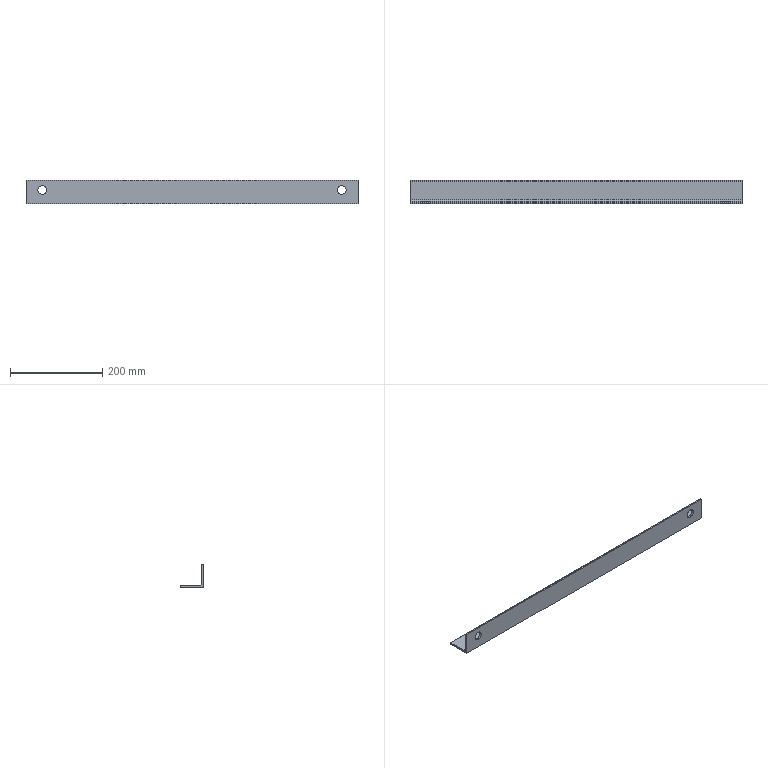Part | STEP file | 休息台角钢1_Default<As Machined> | 1 solid | 15 faces | box 721.5 x 50 x 50 mm | volume 278924 mm3 | plane 8 | cylinder 7 | commonest cylinder face diameters 19 x4 2.66 x2 11 x1
STEP:
#1=CARTESIAN_POINT('',(0.,0.,0.));
#2=DIRECTION('',(0.,0.,1.));
#3=DIRECTION('',(1.,0.,0.));
#4=AXIS2_PLACEMENT_3D('',#1,#2,#3);
#5=CARTESIAN_POINT('',(-325.75,0.,38.585));
#6=VERTEX_POINT('',#5);
#7=CARTESIAN_POINT('',(-325.75,4.,38.585));
#8=VERTEX_POINT('',#7);
#9=CARTESIAN_POINT('',(-325.75,-6.,38.585));
#10=DIRECTION('',(0.,1.,0.));
#11=VECTOR('',#10,1.);
#12=LINE('',#9,#11);
#13=CARTESIAN_POINT('',(-325.75,-6.,29.085));
#14=DIRECTION('',(0.,1.,0.));
#15=DIRECTION('',(0.,0.,1.));
#16=AXIS2_PLACEMENT_3D('',#13,#14,#15);
#17=CYLINDRICAL_SURFACE('',#16,9.5);
#18=CARTESIAN_POINT('',(6.283,0.));
#19=DIRECTION('',(0.,1.));
#20=VECTOR('',#19,1.);
#21=LINE('',#18,#20);
#22=(GEOMETRIC_REPRESENTATION_CONTEXT(2)PARAMETRIC_REPRESENTATION_CONTEXT()REPRESENTATION_CONTEXT('',''));
#23=DEFINITIONAL_REPRESENTATION('',(#21),#22);
#24=PCURVE('',#17,#23);
#25=CARTESIAN_POINT('',(-325.75,-6.,29.085));
#26=DIRECTION('',(0.,1.,0.));
#27=DIRECTION('',(0.,0.,1.));
#28=AXIS2_PLACEMENT_3D('',#25,#26,#27);
#29=CYLINDRICAL_SURFACE('',#28,9.5);
#30=CARTESIAN_POINT('',(0.,0.));
#31=DIRECTION('',(0.,1.));
#32=VECTOR('',#31,1.);
#33=LINE('',#30,#32);
#34=(GEOMETRIC_REPRESENTATION_CONTEXT(2)PARAMETRIC_REPRESENTATION_CONTEXT()REPRESENTATION_CONTEXT('',''));
#35=DEFINITIONAL_REPRESENTATION('',(#33),#34);
#36=PCURVE('',#29,#35);
#37=SURFACE_CURVE('',#12,(#24,#36),.PCURVE_S1.);
#38=EDGE_CURVE('',#6,#8,#37,.T.);
#39=ORIENTED_EDGE('',*,*,#38,.T.);
#40=CARTESIAN_POINT('',(-325.75,4.,19.585));
#41=VERTEX_POINT('',#40);
#42=CARTESIAN_POINT('',(-325.75,4.,29.085));
#43=DIRECTION('',(0.,1.,0.));
#44=DIRECTION('',(0.,0.,1.));
#45=AXIS2_PLACEMENT_3D('',#42,#43,#44);
#46=CIRCLE('',#45,9.5);
#47=CARTESIAN_POINT('',(0.,10.));
#48=DIRECTION('',(1.,0.));
#49=VECTOR('',#48,1.);
#50=LINE('',#47,#49);
#51=(GEOMETRIC_REPRESENTATION_CONTEXT(2)PARAMETRIC_REPRESENTATION_CONTEXT()REPRESENTATION_CONTEXT('',''));
#52=DEFINITIONAL_REPRESENTATION('',(#50),#51);
#53=PCURVE('',#17,#52);
#54=CARTESIAN_POINT('',(360.75,4.,48.67));
#55=DIRECTION('',(0.,-1.,0.));
#56=DIRECTION('',(1.,0.,0.));
#57=AXIS2_PLACEMENT_3D('',#54,#55,#56);
#58=PLANE('',#57);
#59=CARTESIAN_POINT('',(-686.5,-10.085));
#60=CARTESIAN_POINT('',(-670.046,-10.085));
#61=CARTESIAN_POINT('',(-678.273,-24.335));
#62=CARTESIAN_POINT('',(-686.5,-38.585));
#63=CARTESIAN_POINT('',(-694.727,-24.335));
#64=CARTESIAN_POINT('',(-702.954,-10.085));
#65=CARTESIAN_POINT('',(-686.5,-10.085));
#66=(BOUNDED_CURVE()B_SPLINE_CURVE(2,(#59,#60,#61,#62,#63,#64,#65),.UNSPECIFIED.,.T.,.F.)B_SPLINE_CURVE_WITH_KNOTS((1,2,2,2,2,1),(-2.094,0.,2.094,4.189,6.283,8.378),.UNSPECIFIED.)CURVE()GEOMETRIC_REPRESENTATION_ITEM()RATIONAL_B_SPLINE_CURVE((1.,0.5,1.,0.5,1.,0.5,1.))REPRESENTATION_ITEM(''));
#67=(GEOMETRIC_REPRESENTATION_CONTEXT(2)PARAMETRIC_REPRESENTATION_CONTEXT()REPRESENTATION_CONTEXT('',''));
#68=DEFINITIONAL_REPRESENTATION('',(#66),#67);
#69=PCURVE('',#58,#68);
#70=SURFACE_CURVE('',#46,(#53,#69),.PCURVE_S1.);
#71=EDGE_CURVE('',#41,#8,#70,.T.);
#72=ORIENTED_EDGE('',*,*,#71,.F.);
#73=CARTESIAN_POINT('',(-325.75,0.,19.585));
#74=VERTEX_POINT('',#73);
#75=CARTESIAN_POINT('',(-325.75,-6.,19.585));
#76=DIRECTION('',(0.,1.,0.));
#77=VECTOR('',#76,1.);
#78=LINE('',#75,#77);
#79=CARTESIAN_POINT('',(3.142,0.));
#80=DIRECTION('',(0.,1.));
#81=VECTOR('',#80,1.);
#82=LINE('',#79,#81);
#83=(GEOMETRIC_REPRESENTATION_CONTEXT(2)PARAMETRIC_REPRESENTATION_CONTEXT()REPRESENTATION_CONTEXT('',''));
#84=DEFINITIONAL_REPRESENTATION('',(#82),#83);
#85=PCURVE('',#17,#84);
#86=CARTESIAN_POINT('',(3.142,0.));
#87=DIRECTION('',(0.,1.));
#88=VECTOR('',#87,1.);
#89=LINE('',#86,#88);
#90=(GEOMETRIC_REPRESENTATION_CONTEXT(2)PARAMETRIC_REPRESENTATION_CONTEXT()REPRESENTATION_CONTEXT('',''));
#91=DEFINITIONAL_REPRESENTATION('',(#89),#90);
#92=PCURVE('',#29,#91);
#93=SURFACE_CURVE('',#78,(#85,#92),.PCURVE_S1.);
#94=EDGE_CURVE('',#74,#41,#93,.T.);
#95=ORIENTED_EDGE('',*,*,#94,.F.);
#96=CARTESIAN_POINT('',(-325.75,0.,29.085));
#97=DIRECTION('',(0.,1.,0.));
#98=DIRECTION('',(-1.,0.,0.));
#99=AXIS2_PLACEMENT_3D('',#96,#97,#98);
#100=CIRCLE('',#99,9.5);
#101=CARTESIAN_POINT('',(-1.571,6.));
#102=DIRECTION('',(1.,0.));
#103=VECTOR('',#102,1.);
#104=LINE('',#101,#103);
#105=(GEOMETRIC_REPRESENTATION_CONTEXT(2)PARAMETRIC_REPRESENTATION_CONTEXT()REPRESENTATION_CONTEXT('',''));
#106=DEFINITIONAL_REPRESENTATION('',(#104),#105);
#107=PCURVE('',#17,#106);
#108=CARTESIAN_POINT('',(360.75,0.,50.));
#109=DIRECTION('',(0.,1.,0.));
#110=DIRECTION('',(-1.,0.,0.));
#111=AXIS2_PLACEMENT_3D('',#108,#109,#110);
#112=PLANE('',#111);
#113=CARTESIAN_POINT('',(686.5,-20.915));
#114=DIRECTION('',(1.,0.));
#115=AXIS2_PLACEMENT_2D('',#113,#114);
#116=CIRCLE('',#115,9.5);
#117=(GEOMETRIC_REPRESENTATION_CONTEXT(2)PARAMETRIC_REPRESENTATION_CONTEXT()REPRESENTATION_CONTEXT('',''));
#118=DEFINITIONAL_REPRESENTATION('',(#116),#117);
#119=PCURVE('',#112,#118);
#120=SURFACE_CURVE('',#100,(#107,#119),.PCURVE_S1.);
#121=EDGE_CURVE('',#74,#6,#120,.T.);
#122=ORIENTED_EDGE('',*,*,#121,.T.);
#123=EDGE_LOOP('',(#39,#72,#95,#122));
#124=FACE_BOUND('',#123,.F.);
#125=ADVANCED_FACE('',(#124),#17,.F.);
#126=CARTESIAN_POINT('',(325.75,0.,38.585));
#127=VERTEX_POINT('',#126);
#128=CARTESIAN_POINT('',(325.75,4.,38.585));
#129=VERTEX_POINT('',#128);
#130=CARTESIAN_POINT('',(325.75,-6.,38.585));
#131=DIRECTION('',(0.,1.,0.));
#132=VECTOR('',#131,1.);
#133=LINE('',#130,#132);
#134=CARTESIAN_POINT('',(325.75,-6.,29.085));
#135=DIRECTION('',(0.,1.,0.));
#136=DIRECTION('',(0.,0.,1.));
#137=AXIS2_PLACEMENT_3D('',#134,#135,#136);
#138=CYLINDRICAL_SURFACE('',#137,9.5);
#139=CARTESIAN_POINT('',(6.283,0.));
#140=DIRECTION('',(0.,1.));
#141=VECTOR('',#140,1.);
#142=LINE('',#139,#141);
#143=(GEOMETRIC_REPRESENTATION_CONTEXT(2)PARAMETRIC_REPRESENTATION_CONTEXT()REPRESENTATION_CONTEXT('',''));
#144=DEFINITIONAL_REPRESENTATION('',(#142),#143);
#145=PCURVE('',#138,#144);
#146=CARTESIAN_POINT('',(325.75,-6.,29.085));
#147=DIRECTION('',(0.,1.,0.));
#148=DIRECTION('',(0.,0.,1.));
#149=AXIS2_PLACEMENT_3D('',#146,#147,#148);
#150=CYLINDRICAL_SURFACE('',#149,9.5);
#151=CARTESIAN_POINT('',(0.,0.));
#152=DIRECTION('',(0.,1.));
#153=VECTOR('',#152,1.);
#154=LINE('',#151,#153);
#155=(GEOMETRIC_REPRESENTATION_CONTEXT(2)PARAMETRIC_REPRESENTATION_CONTEXT()REPRESENTATION_CONTEXT('',''));
#156=DEFINITIONAL_REPRESENTATION('',(#154),#155);
#157=PCURVE('',#150,#156);
#158=SURFACE_CURVE('',#133,(#145,#157),.PCURVE_S1.);
#159=EDGE_CURVE('',#127,#129,#158,.T.);
#160=ORIENTED_EDGE('',*,*,#159,.T.);
#161=CARTESIAN_POINT('',(325.75,4.,19.585));
#162=VERTEX_POINT('',#161);
#163=CARTESIAN_POINT('',(325.75,4.,29.085));
#164=DIRECTION('',(0.,1.,0.));
#165=DIRECTION('',(0.,0.,-1.));
#166=AXIS2_PLACEMENT_3D('',#163,#164,#165);
#167=CIRCLE('',#166,9.5);
#168=CARTESIAN_POINT('',(3.142,10.));
#169=DIRECTION('',(1.,0.));
#170=VECTOR('',#169,1.);
#171=LINE('',#168,#170);
#172=(GEOMETRIC_REPRESENTATION_CONTEXT(2)PARAMETRIC_REPRESENTATION_CONTEXT()REPRESENTATION_CONTEXT('',''));
#173=DEFINITIONAL_REPRESENTATION('',(#171),#172);
#174=PCURVE('',#138,#173);
#175=CARTESIAN_POINT('',(-35.,-29.085));
#176=CARTESIAN_POINT('',(-51.454,-29.085));
#177=CARTESIAN_POINT('',(-43.227,-14.835));
#178=CARTESIAN_POINT('',(-35.,-0.585));
#179=CARTESIAN_POINT('',(-26.773,-14.835));
#180=CARTESIAN_POINT('',(-18.546,-29.085));
#181=CARTESIAN_POINT('',(-35.,-29.085));
#182=(BOUNDED_CURVE()B_SPLINE_CURVE(2,(#175,#176,#177,#178,#179,#180,#181),.UNSPECIFIED.,.T.,.F.)B_SPLINE_CURVE_WITH_KNOTS((1,2,2,2,2,1),(-2.094,0.,2.094,4.189,6.283,8.378),.UNSPECIFIED.)CURVE()GEOMETRIC_REPRESENTATION_ITEM()RATIONAL_B_SPLINE_CURVE((1.,0.5,1.,0.5,1.,0.5,1.))REPRESENTATION_ITEM(''));
#183=(GEOMETRIC_REPRESENTATION_CONTEXT(2)PARAMETRIC_REPRESENTATION_CONTEXT()REPRESENTATION_CONTEXT('',''));
#184=DEFINITIONAL_REPRESENTATION('',(#182),#183);
#185=PCURVE('',#58,#184);
#186=SURFACE_CURVE('',#167,(#174,#185),.PCURVE_S1.);
#187=EDGE_CURVE('',#162,#129,#186,.T.);
#188=ORIENTED_EDGE('',*,*,#187,.F.);
#189=CARTESIAN_POINT('',(325.75,0.,19.585));
#190=VERTEX_POINT('',#189);
#191=CARTESIAN_POINT('',(325.75,-6.,19.585));
#192=DIRECTION('',(0.,1.,0.));
#193=VECTOR('',#192,1.);
#194=LINE('',#191,#193);
#195=CARTESIAN_POINT('',(3.142,0.));
#196=DIRECTION('',(0.,1.));
#197=VECTOR('',#196,1.);
#198=LINE('',#195,#197);
#199=(GEOMETRIC_REPRESENTATION_CONTEXT(2)PARAMETRIC_REPRESENTATION_CONTEXT()REPRESENTATION_CONTEXT('',''));
#200=DEFINITIONAL_REPRESENTATION('',(#198),#199);
#201=PCURVE('',#138,#200);
#202=CARTESIAN_POINT('',(3.142,0.));
#203=DIRECTION('',(0.,1.));
#204=VECTOR('',#203,1.);
#205=LINE('',#202,#204);
#206=(GEOMETRIC_REPRESENTATION_CONTEXT(2)PARAMETRIC_REPRESENTATION_CONTEXT()REPRESENTATION_CONTEXT('',''));
#207=DEFINITIONAL_REPRESENTATION('',(#205),#206);
#208=PCURVE('',#150,#207);
#209=SURFACE_CURVE('',#194,(#201,#208),.PCURVE_S1.);
#210=EDGE_CURVE('',#190,#162,#209,.T.);
#211=ORIENTED_EDGE('',*,*,#210,.F.);
#212=CARTESIAN_POINT('',(325.75,0.,29.085));
#213=DIRECTION('',(0.,1.,0.));
#214=DIRECTION('',(-1.,0.,0.));
#215=AXIS2_PLACEMENT_3D('',#212,#213,#214);
#216=CIRCLE('',#215,9.5);
#217=CARTESIAN_POINT('',(-1.571,6.));
#218=DIRECTION('',(1.,0.));
#219=VECTOR('',#218,1.);
#220=LINE('',#217,#219);
#221=(GEOMETRIC_REPRESENTATION_CONTEXT(2)PARAMETRIC_REPRESENTATION_CONTEXT()REPRESENTATION_CONTEXT('',''));
#222=DEFINITIONAL_REPRESENTATION('',(#220),#221);
#223=PCURVE('',#138,#222);
#224=CARTESIAN_POINT('',(35.,-20.915));
#225=DIRECTION('',(1.,0.));
#226=AXIS2_PLACEMENT_2D('',#224,#225);
#227=CIRCLE('',#226,9.5);
#228=(GEOMETRIC_REPRESENTATION_CONTEXT(2)PARAMETRIC_REPRESENTATION_CONTEXT()REPRESENTATION_CONTEXT('',''));
#229=DEFINITIONAL_REPRESENTATION('',(#227),#228);
#230=PCURVE('',#112,#229);
#231=SURFACE_CURVE('',#216,(#223,#230),.PCURVE_S1.);
#232=EDGE_CURVE('',#190,#127,#231,.T.);
#233=ORIENTED_EDGE('',*,*,#232,.T.);
#234=EDGE_LOOP('',(#160,#188,#211,#233));
#235=FACE_BOUND('',#234,.F.);
#236=ADVANCED_FACE('',(#235),#138,.F.);
#237=CARTESIAN_POINT('',(-360.75,50.,2.67));
#238=VERTEX_POINT('',#237);
#239=CARTESIAN_POINT('',(-360.75,48.67,4.));
#240=VERTEX_POINT('',#239);
#241=CARTESIAN_POINT('',(-360.75,48.67,2.67));
#242=DIRECTION('',(1.,0.,0.));
#243=DIRECTION('',(0.,1.,0.));
#244=AXIS2_PLACEMENT_3D('',#241,#242,#243);
#245=CIRCLE('',#244,1.33);
#246=CARTESIAN_POINT('',(360.75,48.67,2.67));
#247=DIRECTION('',(-1.,0.,0.));
#248=DIRECTION('',(0.,-1.,0.));
#249=AXIS2_PLACEMENT_3D('',#246,#247,#248);
#250=CYLINDRICAL_SURFACE('',#249,1.33);
#251=CARTESIAN_POINT('',(3.142,721.5));
#252=DIRECTION('',(-1.,0.));
#253=VECTOR('',#252,1.);
#254=LINE('',#251,#253);
#255=(GEOMETRIC_REPRESENTATION_CONTEXT(2)PARAMETRIC_REPRESENTATION_CONTEXT()REPRESENTATION_CONTEXT('',''));
#256=DEFINITIONAL_REPRESENTATION('',(#254),#255);
#257=PCURVE('',#250,#256);
#258=CARTESIAN_POINT('',(-360.75,48.67,2.67));
#259=DIRECTION('',(1.,0.,0.));
#260=DIRECTION('',(0.,1.,0.));
#261=AXIS2_PLACEMENT_3D('',#258,#259,#260);
#262=PLANE('',#261);
#263=CARTESIAN_POINT('',(0.,0.));
#264=DIRECTION('',(1.,0.));
#265=AXIS2_PLACEMENT_2D('',#263,#264);
#266=CIRCLE('',#265,1.33);
#267=(GEOMETRIC_REPRESENTATION_CONTEXT(2)PARAMETRIC_REPRESENTATION_CONTEXT()REPRESENTATION_CONTEXT('',''));
#268=DEFINITIONAL_REPRESENTATION('',(#266),#267);
#269=PCURVE('',#262,#268);
#270=SURFACE_CURVE('',#245,(#257,#269),.PCURVE_S1.);
#271=EDGE_CURVE('',#238,#240,#270,.T.);
#272=ORIENTED_EDGE('',*,*,#271,.T.);
#273=CARTESIAN_POINT('',(360.75,48.67,4.));
#274=VERTEX_POINT('',#273);
#275=CARTESIAN_POINT('',(360.75,48.67,4.));
#276=DIRECTION('',(-1.,0.,0.));
#277=VECTOR('',#276,1.);
#278=LINE('',#275,#277);
#279=CARTESIAN_POINT('',(1.571,0.));
#280=DIRECTION('',(0.,1.));
#281=VECTOR('',#280,1.);
#282=LINE('',#279,#281);
#283=(GEOMETRIC_REPRESENTATION_CONTEXT(2)PARAMETRIC_REPRESENTATION_CONTEXT()REPRESENTATION_CONTEXT('',''));
#284=DEFINITIONAL_REPRESENTATION('',(#282),#283);
#285=PCURVE('',#250,#284);
#286=CARTESIAN_POINT('',(360.75,9.5,4.));
#287=DIRECTION('',(0.,0.,-1.));
#288=DIRECTION('',(-1.,0.,0.));
#289=AXIS2_PLACEMENT_3D('',#286,#287,#288);
#290=PLANE('',#289);
#291=CARTESIAN_POINT('',(0.,39.17));
#292=DIRECTION('',(1.,0.));
#293=VECTOR('',#292,1.);
#294=LINE('',#291,#293);
#295=(GEOMETRIC_REPRESENTATION_CONTEXT(2)PARAMETRIC_REPRESENTATION_CONTEXT()REPRESENTATION_CONTEXT('',''));
#296=DEFINITIONAL_REPRESENTATION('',(#294),#295);
#297=PCURVE('',#290,#296);
#298=SURFACE_CURVE('',#278,(#285,#297),.PCURVE_S1.);
#299=EDGE_CURVE('',#274,#240,#298,.T.);
#300=ORIENTED_EDGE('',*,*,#299,.F.);
#301=CARTESIAN_POINT('',(360.75,50.,2.67));
#302=VERTEX_POINT('',#301);
#303=CARTESIAN_POINT('',(360.75,48.67,2.67));
#304=DIRECTION('',(1.,0.,0.));
#305=DIRECTION('',(0.,1.,0.));
#306=AXIS2_PLACEMENT_3D('',#303,#304,#305);
#307=CIRCLE('',#306,1.33);
#308=CARTESIAN_POINT('',(3.142,0.));
#309=DIRECTION('',(-1.,0.));
#310=VECTOR('',#309,1.);
#311=LINE('',#308,#310);
#312=(GEOMETRIC_REPRESENTATION_CONTEXT(2)PARAMETRIC_REPRESENTATION_CONTEXT()REPRESENTATION_CONTEXT('',''));
#313=DEFINITIONAL_REPRESENTATION('',(#311),#312);
#314=PCURVE('',#250,#313);
#315=CARTESIAN_POINT('',(360.75,48.67,2.67));
#316=DIRECTION('',(1.,0.,0.));
#317=DIRECTION('',(0.,1.,0.));
#318=AXIS2_PLACEMENT_3D('',#315,#316,#317);
#319=PLANE('',#318);
#320=CARTESIAN_POINT('',(0.,0.));
#321=DIRECTION('',(1.,0.));
#322=AXIS2_PLACEMENT_2D('',#320,#321);
#323=CIRCLE('',#322,1.33);
#324=(GEOMETRIC_REPRESENTATION_CONTEXT(2)PARAMETRIC_REPRESENTATION_CONTEXT()REPRESENTATION_CONTEXT('',''));
#325=DEFINITIONAL_REPRESENTATION('',(#323),#324);
#326=PCURVE('',#319,#325);
#327=SURFACE_CURVE('',#307,(#314,#326),.PCURVE_S1.);
#328=EDGE_CURVE('',#302,#274,#327,.T.);
#329=ORIENTED_EDGE('',*,*,#328,.F.);
#330=CARTESIAN_POINT('',(360.75,50.,2.67));
#331=DIRECTION('',(-1.,0.,0.));
#332=VECTOR('',#331,1.);
#333=LINE('',#330,#332);
#334=CARTESIAN_POINT('',(3.142,0.));
#335=DIRECTION('',(0.,1.));
#336=VECTOR('',#335,1.);
#337=LINE('',#334,#336);
#338=(GEOMETRIC_REPRESENTATION_CONTEXT(2)PARAMETRIC_REPRESENTATION_CONTEXT()REPRESENTATION_CONTEXT('',''));
#339=DEFINITIONAL_REPRESENTATION('',(#337),#338);
#340=PCURVE('',#250,#339);
#341=CARTESIAN_POINT('',(360.75,50.,2.67));
#342=DIRECTION('',(0.,-1.,0.));
#343=DIRECTION('',(1.,0.,0.));
#344=AXIS2_PLACEMENT_3D('',#341,#342,#343);
#345=PLANE('',#344);
#346=CARTESIAN_POINT('',(0.,0.));
#347=DIRECTION('',(-1.,0.));
#348=VECTOR('',#347,1.);
#349=LINE('',#346,#348);
#350=(GEOMETRIC_REPRESENTATION_CONTEXT(2)PARAMETRIC_REPRESENTATION_CONTEXT()REPRESENTATION_CONTEXT('',''));
#351=DEFINITIONAL_REPRESENTATION('',(#349),#350);
#352=PCURVE('',#345,#351);
#353=SURFACE_CURVE('',#333,(#340,#352),.PCURVE_S1.);
#354=EDGE_CURVE('',#302,#238,#353,.T.);
#355=ORIENTED_EDGE('',*,*,#354,.T.);
#356=EDGE_LOOP('',(#272,#300,#329,#355));
#357=FACE_BOUND('',#356,.T.);
#358=ADVANCED_FACE('',(#357),#250,.T.);
#359=CARTESIAN_POINT('',(-360.75,9.5,4.));
#360=VERTEX_POINT('',#359);
#361=CARTESIAN_POINT('',(-360.75,9.5,4.));
#362=DIRECTION('',(0.,-1.,0.));
#363=VECTOR('',#362,1.);
#364=LINE('',#361,#363);
#365=CARTESIAN_POINT('',(721.5,0.));
#366=DIRECTION('',(0.,-1.));
#367=VECTOR('',#366,1.);
#368=LINE('',#365,#367);
#369=(GEOMETRIC_REPRESENTATION_CONTEXT(2)PARAMETRIC_REPRESENTATION_CONTEXT()REPRESENTATION_CONTEXT('',''));
#370=DEFINITIONAL_REPRESENTATION('',(#368),#369);
#371=PCURVE('',#290,#370);
#372=CARTESIAN_POINT('',(-39.17,1.33));
#373=DIRECTION('',(-1.,0.));
#374=VECTOR('',#373,1.);
#375=LINE('',#372,#374);
#376=(GEOMETRIC_REPRESENTATION_CONTEXT(2)PARAMETRIC_REPRESENTATION_CONTEXT()REPRESENTATION_CONTEXT('',''));
#377=DEFINITIONAL_REPRESENTATION('',(#375),#376);
#378=PCURVE('',#262,#377);
#379=SURFACE_CURVE('',#364,(#371,#378),.PCURVE_S1.);
#380=EDGE_CURVE('',#240,#360,#379,.T.);
#381=ORIENTED_EDGE('',*,*,#380,.T.);
#382=CARTESIAN_POINT('',(360.75,9.5,4.));
#383=VERTEX_POINT('',#382);
#384=CARTESIAN_POINT('',(360.75,9.5,4.));
#385=DIRECTION('',(-1.,0.,0.));
#386=VECTOR('',#385,1.);
#387=LINE('',#384,#386);
#388=CARTESIAN_POINT('',(0.,0.));
#389=DIRECTION('',(1.,0.));
#390=VECTOR('',#389,1.);
#391=LINE('',#388,#390);
#392=(GEOMETRIC_REPRESENTATION_CONTEXT(2)PARAMETRIC_REPRESENTATION_CONTEXT()REPRESENTATION_CONTEXT('',''));
#393=DEFINITIONAL_REPRESENTATION('',(#391),#392);
#394=PCURVE('',#290,#393);
#395=CARTESIAN_POINT('',(360.75,9.5,9.5));
#396=DIRECTION('',(-1.,0.,0.));
#397=DIRECTION('',(0.,-1.,0.));
#398=AXIS2_PLACEMENT_3D('',#395,#396,#397);
#399=CYLINDRICAL_SURFACE('',#398,5.5);
#400=CARTESIAN_POINT('',(4.712,0.));
#401=DIRECTION('',(0.,1.));
#402=VECTOR('',#401,1.);
#403=LINE('',#400,#402);
#404=(GEOMETRIC_REPRESENTATION_CONTEXT(2)PARAMETRIC_REPRESENTATION_CONTEXT()REPRESENTATION_CONTEXT('',''));
#405=DEFINITIONAL_REPRESENTATION('',(#403),#404);
#406=PCURVE('',#399,#405);
#407=SURFACE_CURVE('',#387,(#394,#406),.PCURVE_S1.);
#408=EDGE_CURVE('',#383,#360,#407,.T.);
#409=ORIENTED_EDGE('',*,*,#408,.F.);
#410=CARTESIAN_POINT('',(360.75,9.5,4.));
#411=DIRECTION('',(0.,-1.,0.));
#412=VECTOR('',#411,1.);
#413=LINE('',#410,#412);
#414=CARTESIAN_POINT('',(0.,0.));
#415=DIRECTION('',(0.,-1.));
#416=VECTOR('',#415,1.);
#417=LINE('',#414,#416);
#418=(GEOMETRIC_REPRESENTATION_CONTEXT(2)PARAMETRIC_REPRESENTATION_CONTEXT()REPRESENTATION_CONTEXT('',''));
#419=DEFINITIONAL_REPRESENTATION('',(#417),#418);
#420=PCURVE('',#290,#419);
#421=CARTESIAN_POINT('',(-39.17,1.33));
#422=DIRECTION('',(-1.,0.));
#423=VECTOR('',#422,1.);
#424=LINE('',#421,#423);
#425=(GEOMETRIC_REPRESENTATION_CONTEXT(2)PARAMETRIC_REPRESENTATION_CONTEXT()REPRESENTATION_CONTEXT('',''));
#426=DEFINITIONAL_REPRESENTATION('',(#424),#425);
#427=PCURVE('',#319,#426);
#428=SURFACE_CURVE('',#413,(#420,#427),.PCURVE_S1.);
#429=EDGE_CURVE('',#274,#383,#428,.T.);
#430=ORIENTED_EDGE('',*,*,#429,.F.);
#431=ORIENTED_EDGE('',*,*,#299,.T.);
#432=EDGE_LOOP('',(#381,#409,#430,#431));
#433=FACE_BOUND('',#432,.T.);
#434=ADVANCED_FACE('',(#433),#290,.F.);
#435=ORIENTED_EDGE('',*,*,#408,.F.);
#436=CARTESIAN_POINT('',(360.75,4.,9.5));
#437=VERTEX_POINT('',#436);
#438=CARTESIAN_POINT('',(360.75,9.5,9.5));
#439=DIRECTION('',(-1.,0.,0.));
#440=DIRECTION('',(0.,1.,0.));
#441=AXIS2_PLACEMENT_3D('',#438,#439,#440);
#442=CIRCLE('',#441,5.5);
#443=CARTESIAN_POINT('',(3.142,0.));
#444=DIRECTION('',(1.,0.));
#445=VECTOR('',#444,1.);
#446=LINE('',#443,#445);
#447=(GEOMETRIC_REPRESENTATION_CONTEXT(2)PARAMETRIC_REPRESENTATION_CONTEXT()REPRESENTATION_CONTEXT('',''));
#448=DEFINITIONAL_REPRESENTATION('',(#446),#447);
#449=PCURVE('',#399,#448);
#450=CARTESIAN_POINT('',(-33.67,6.83));
#451=CARTESIAN_POINT('',(-33.67,-2.696));
#452=CARTESIAN_POINT('',(-41.92,2.067));
#453=CARTESIAN_POINT('',(-50.17,6.83));
#454=CARTESIAN_POINT('',(-41.92,11.593));
#455=CARTESIAN_POINT('',(-33.67,16.356));
#456=CARTESIAN_POINT('',(-33.67,6.83));
#457=(BOUNDED_CURVE()B_SPLINE_CURVE(2,(#450,#451,#452,#453,#454,#455,#456),.UNSPECIFIED.,.T.,.F.)B_SPLINE_CURVE_WITH_KNOTS((1,2,2,2,2,1),(-2.094,0.,2.094,4.189,6.283,8.378),.UNSPECIFIED.)CURVE()GEOMETRIC_REPRESENTATION_ITEM()RATIONAL_B_SPLINE_CURVE((1.,0.5,1.,0.5,1.,0.5,1.))REPRESENTATION_ITEM(''));
#458=(GEOMETRIC_REPRESENTATION_CONTEXT(2)PARAMETRIC_REPRESENTATION_CONTEXT()REPRESENTATION_CONTEXT('',''));
#459=DEFINITIONAL_REPRESENTATION('',(#457),#458);
#460=PCURVE('',#319,#459);
#461=SURFACE_CURVE('',#442,(#449,#460),.PCURVE_S1.);
#462=EDGE_CURVE('',#383,#437,#461,.T.);
#463=ORIENTED_EDGE('',*,*,#462,.T.);
#464=CARTESIAN_POINT('',(-360.75,4.,9.5));
#465=VERTEX_POINT('',#464);
#466=CARTESIAN_POINT('',(360.75,4.,9.5));
#467=DIRECTION('',(-1.,0.,0.));
#468=VECTOR('',#467,1.);
#469=LINE('',#466,#468);
#470=CARTESIAN_POINT('',(6.283,0.));
#471=DIRECTION('',(0.,1.));
#472=VECTOR('',#471,1.);
#473=LINE('',#470,#472);
#474=(GEOMETRIC_REPRESENTATION_CONTEXT(2)PARAMETRIC_REPRESENTATION_CONTEXT()REPRESENTATION_CONTEXT('',''));
#475=DEFINITIONAL_REPRESENTATION('',(#473),#474);
#476=PCURVE('',#399,#475);
#477=CARTESIAN_POINT('',(0.,-39.17));
#478=DIRECTION('',(-1.,0.));
#479=VECTOR('',#478,1.);
#480=LINE('',#477,#479);
#481=(GEOMETRIC_REPRESENTATION_CONTEXT(2)PARAMETRIC_REPRESENTATION_CONTEXT()REPRESENTATION_CONTEXT('',''));
#482=DEFINITIONAL_REPRESENTATION('',(#480),#481);
#483=PCURVE('',#58,#482);
#484=SURFACE_CURVE('',#469,(#476,#483),.PCURVE_S1.);
#485=EDGE_CURVE('',#437,#465,#484,.T.);
#486=ORIENTED_EDGE('',*,*,#485,.T.);
#487=CARTESIAN_POINT('',(-360.75,9.5,9.5));
#488=DIRECTION('',(-1.,0.,0.));
#489=DIRECTION('',(0.,1.,0.));
#490=AXIS2_PLACEMENT_3D('',#487,#488,#489);
#491=CIRCLE('',#490,5.5);
#492=CARTESIAN_POINT('',(3.142,721.5));
#493=DIRECTION('',(1.,0.));
#494=VECTOR('',#493,1.);
#495=LINE('',#492,#494);
#496=(GEOMETRIC_REPRESENTATION_CONTEXT(2)PARAMETRIC_REPRESENTATION_CONTEXT()REPRESENTATION_CONTEXT('',''));
#497=DEFINITIONAL_REPRESENTATION('',(#495),#496);
#498=PCURVE('',#399,#497);
#499=CARTESIAN_POINT('',(-33.67,6.83));
#500=CARTESIAN_POINT('',(-33.67,-2.696));
#501=CARTESIAN_POINT('',(-41.92,2.067));
#502=CARTESIAN_POINT('',(-50.17,6.83));
#503=CARTESIAN_POINT('',(-41.92,11.593));
#504=CARTESIAN_POINT('',(-33.67,16.356));
#505=CARTESIAN_POINT('',(-33.67,6.83));
#506=(BOUNDED_CURVE()B_SPLINE_CURVE(2,(#499,#500,#501,#502,#503,#504,#505),.UNSPECIFIED.,.T.,.F.)B_SPLINE_CURVE_WITH_KNOTS((1,2,2,2,2,1),(-2.094,0.,2.094,4.189,6.283,8.378),.UNSPECIFIED.)CURVE()GEOMETRIC_REPRESENTATION_ITEM()RATIONAL_B_SPLINE_CURVE((1.,0.5,1.,0.5,1.,0.5,1.))REPRESENTATION_ITEM(''));
#507=(GEOMETRIC_REPRESENTATION_CONTEXT(2)PARAMETRIC_REPRESENTATION_CONTEXT()REPRESENTATION_CONTEXT('',''));
#508=DEFINITIONAL_REPRESENTATION('',(#506),#507);
#509=PCURVE('',#262,#508);
#510=SURFACE_CURVE('',#491,(#498,#509),.PCURVE_S1.);
#511=EDGE_CURVE('',#360,#465,#510,.T.);
#512=ORIENTED_EDGE('',*,*,#511,.F.);
#513=EDGE_LOOP('',(#435,#463,#486,#512));
#514=FACE_BOUND('',#513,.F.);
#515=ADVANCED_FACE('',(#514),#399,.F.);
#516=CARTESIAN_POINT('',(-325.75,4.,29.085));
#517=DIRECTION('',(0.,1.,0.));
#518=DIRECTION('',(0.,0.,1.));
#519=AXIS2_PLACEMENT_3D('',#516,#517,#518);
#520=CIRCLE('',#519,9.5);
#521=CARTESIAN_POINT('',(-686.5,-10.085));
#522=CARTESIAN_POINT('',(-670.046,-10.085));
#523=CARTESIAN_POINT('',(-678.273,-24.335));
#524=CARTESIAN_POINT('',(-686.5,-38.585));
#525=CARTESIAN_POINT('',(-694.727,-24.335));
#526=CARTESIAN_POINT('',(-702.954,-10.085));
#527=CARTESIAN_POINT('',(-686.5,-10.085));
#528=(BOUNDED_CURVE()B_SPLINE_CURVE(2,(#521,#522,#523,#524,#525,#526,#527),.UNSPECIFIED.,.T.,.F.)B_SPLINE_CURVE_WITH_KNOTS((1,2,2,2,2,1),(-2.094,0.,2.094,4.189,6.283,8.378),.UNSPECIFIED.)CURVE()GEOMETRIC_REPRESENTATION_ITEM()RATIONAL_B_SPLINE_CURVE((1.,0.5,1.,0.5,1.,0.5,1.))REPRESENTATION_ITEM(''));
#529=(GEOMETRIC_REPRESENTATION_CONTEXT(2)PARAMETRIC_REPRESENTATION_CONTEXT()REPRESENTATION_CONTEXT('',''));
#530=DEFINITIONAL_REPRESENTATION('',(#528),#529);
#531=PCURVE('',#58,#530);
#532=CARTESIAN_POINT('',(0.,10.));
#533=DIRECTION('',(1.,0.));
#534=VECTOR('',#533,1.);
#535=LINE('',#532,#534);
#536=(GEOMETRIC_REPRESENTATION_CONTEXT(2)PARAMETRIC_REPRESENTATION_CONTEXT()REPRESENTATION_CONTEXT('',''));
#537=DEFINITIONAL_REPRESENTATION('',(#535),#536);
#538=PCURVE('',#29,#537);
#539=SURFACE_CURVE('',#520,(#531,#538),.PCURVE_S1.);
#540=EDGE_CURVE('',#8,#41,#539,.T.);
#541=ORIENTED_EDGE('',*,*,#540,.F.);
#542=ORIENTED_EDGE('',*,*,#71,.F.);
#543=EDGE_LOOP('',(#541,#542));
#544=FACE_BOUND('',#543,.T.);
#545=CARTESIAN_POINT('',(325.75,4.,29.085));
#546=DIRECTION('',(0.,1.,0.));
#547=DIRECTION('',(0.,0.,-1.));
#548=AXIS2_PLACEMENT_3D('',#545,#546,#547);
#549=CIRCLE('',#548,9.5);
#550=CARTESIAN_POINT('',(-35.,-29.085));
#551=CARTESIAN_POINT('',(-51.454,-29.085));
#552=CARTESIAN_POINT('',(-43.227,-14.835));
#553=CARTESIAN_POINT('',(-35.,-0.585));
#554=CARTESIAN_POINT('',(-26.773,-14.835));
#555=CARTESIAN_POINT('',(-18.546,-29.085));
#556=CARTESIAN_POINT('',(-35.,-29.085));
#557=(BOUNDED_CURVE()B_SPLINE_CURVE(2,(#550,#551,#552,#553,#554,#555,#556),.UNSPECIFIED.,.T.,.F.)B_SPLINE_CURVE_WITH_KNOTS((1,2,2,2,2,1),(-2.094,0.,2.094,4.189,6.283,8.378),.UNSPECIFIED.)CURVE()GEOMETRIC_REPRESENTATION_ITEM()RATIONAL_B_SPLINE_CURVE((1.,0.5,1.,0.5,1.,0.5,1.))REPRESENTATION_ITEM(''));
#558=(GEOMETRIC_REPRESENTATION_CONTEXT(2)PARAMETRIC_REPRESENTATION_CONTEXT()REPRESENTATION_CONTEXT('',''));
#559=DEFINITIONAL_REPRESENTATION('',(#557),#558);
#560=PCURVE('',#58,#559);
#561=CARTESIAN_POINT('',(-3.142,10.));
#562=DIRECTION('',(1.,0.));
#563=VECTOR('',#562,1.);
#564=LINE('',#561,#563);
#565=(GEOMETRIC_REPRESENTATION_CONTEXT(2)PARAMETRIC_REPRESENTATION_CONTEXT()REPRESENTATION_CONTEXT('',''));
#566=DEFINITIONAL_REPRESENTATION('',(#564),#565);
#567=PCURVE('',#150,#566);
#568=SURFACE_CURVE('',#549,(#560,#567),.PCURVE_S1.);
#569=EDGE_CURVE('',#129,#162,#568,.T.);
#570=ORIENTED_EDGE('',*,*,#569,.F.);
#571=ORIENTED_EDGE('',*,*,#187,.F.);
#572=EDGE_LOOP('',(#570,#571));
#573=FACE_BOUND('',#572,.T.);
#574=CARTESIAN_POINT('',(-360.75,4.,48.67));
#575=VERTEX_POINT('',#574);
#576=CARTESIAN_POINT('',(-360.75,4.,48.67));
#577=DIRECTION('',(0.,0.,1.));
#578=VECTOR('',#577,1.);
#579=LINE('',#576,#578);
#580=CARTESIAN_POINT('',(-721.5,0.));
#581=DIRECTION('',(0.,1.));
#582=VECTOR('',#581,1.);
#583=LINE('',#580,#582);
#584=(GEOMETRIC_REPRESENTATION_CONTEXT(2)PARAMETRIC_REPRESENTATION_CONTEXT()REPRESENTATION_CONTEXT('',''));
#585=DEFINITIONAL_REPRESENTATION('',(#583),#584);
#586=PCURVE('',#58,#585);
#587=CARTESIAN_POINT('',(-44.67,46.));
#588=DIRECTION('',(0.,1.));
#589=VECTOR('',#588,1.);
#590=LINE('',#587,#589);
#591=(GEOMETRIC_REPRESENTATION_CONTEXT(2)PARAMETRIC_REPRESENTATION_CONTEXT()REPRESENTATION_CONTEXT('',''));
#592=DEFINITIONAL_REPRESENTATION('',(#590),#591);
#593=PCURVE('',#262,#592);
#594=SURFACE_CURVE('',#579,(#586,#593),.PCURVE_S1.);
#595=EDGE_CURVE('',#465,#575,#594,.T.);
#596=ORIENTED_EDGE('',*,*,#595,.T.);
#597=CARTESIAN_POINT('',(360.75,4.,48.67));
#598=VERTEX_POINT('',#597);
#599=CARTESIAN_POINT('',(360.75,4.,48.67));
#600=DIRECTION('',(-1.,0.,0.));
#601=VECTOR('',#600,1.);
#602=LINE('',#599,#601);
#603=CARTESIAN_POINT('',(0.,0.));
#604=DIRECTION('',(-1.,0.));
#605=VECTOR('',#604,1.);
#606=LINE('',#603,#605);
#607=(GEOMETRIC_REPRESENTATION_CONTEXT(2)PARAMETRIC_REPRESENTATION_CONTEXT()REPRESENTATION_CONTEXT('',''));
#608=DEFINITIONAL_REPRESENTATION('',(#606),#607);
#609=PCURVE('',#58,#608);
#610=CARTESIAN_POINT('',(360.75,2.67,48.67));
#611=DIRECTION('',(-1.,0.,0.));
#612=DIRECTION('',(0.,-1.,0.));
#613=AXIS2_PLACEMENT_3D('',#610,#611,#612);
#614=CYLINDRICAL_SURFACE('',#613,1.33);
#615=CARTESIAN_POINT('',(3.142,0.));
#616=DIRECTION('',(0.,1.));
#617=VECTOR('',#616,1.);
#618=LINE('',#615,#617);
#619=(GEOMETRIC_REPRESENTATION_CONTEXT(2)PARAMETRIC_REPRESENTATION_CONTEXT()REPRESENTATION_CONTEXT('',''));
#620=DEFINITIONAL_REPRESENTATION('',(#618),#619);
#621=PCURVE('',#614,#620);
#622=SURFACE_CURVE('',#602,(#609,#621),.PCURVE_S1.);
#623=EDGE_CURVE('',#598,#575,#622,.T.);
#624=ORIENTED_EDGE('',*,*,#623,.F.);
#625=CARTESIAN_POINT('',(360.75,4.,48.67));
#626=DIRECTION('',(0.,0.,1.));
#627=VECTOR('',#626,1.);
#628=LINE('',#625,#627);
#629=CARTESIAN_POINT('',(0.,0.));
#630=DIRECTION('',(0.,1.));
#631=VECTOR('',#630,1.);
#632=LINE('',#629,#631);
#633=(GEOMETRIC_REPRESENTATION_CONTEXT(2)PARAMETRIC_REPRESENTATION_CONTEXT()REPRESENTATION_CONTEXT('',''));
#634=DEFINITIONAL_REPRESENTATION('',(#632),#633);
#635=PCURVE('',#58,#634);
#636=CARTESIAN_POINT('',(-44.67,46.));
#637=DIRECTION('',(0.,1.));
#638=VECTOR('',#637,1.);
#639=LINE('',#636,#638);
#640=(GEOMETRIC_REPRESENTATION_CONTEXT(2)PARAMETRIC_REPRESENTATION_CONTEXT()REPRESENTATION_CONTEXT('',''));
#641=DEFINITIONAL_REPRESENTATION('',(#639),#640);
#642=PCURVE('',#319,#641);
#643=SURFACE_CURVE('',#628,(#635,#642),.PCURVE_S1.);
#644=EDGE_CURVE('',#437,#598,#643,.T.);
#645=ORIENTED_EDGE('',*,*,#644,.F.);
#646=ORIENTED_EDGE('',*,*,#485,.T.);
#647=EDGE_LOOP('',(#596,#624,#645,#646));
#648=FACE_BOUND('',#647,.T.);
#649=ADVANCED_FACE('',(#544,#573,#648),#58,.F.);
#650=CARTESIAN_POINT('',(-360.75,2.67,50.));
#651=VERTEX_POINT('',#650);
#652=CARTESIAN_POINT('',(-360.75,2.67,48.67));
#653=DIRECTION('',(1.,0.,0.));
#654=DIRECTION('',(0.,1.,0.));
#655=AXIS2_PLACEMENT_3D('',#652,#653,#654);
#656=CIRCLE('',#655,1.33);
#657=CARTESIAN_POINT('',(3.142,721.5));
#658=DIRECTION('',(-1.,0.));
#659=VECTOR('',#658,1.);
#660=LINE('',#657,#659);
#661=(GEOMETRIC_REPRESENTATION_CONTEXT(2)PARAMETRIC_REPRESENTATION_CONTEXT()REPRESENTATION_CONTEXT('',''));
#662=DEFINITIONAL_REPRESENTATION('',(#660),#661);
#663=PCURVE('',#614,#662);
#664=CARTESIAN_POINT('',(-46.,46.));
#665=DIRECTION('',(1.,0.));
#666=AXIS2_PLACEMENT_2D('',#664,#665);
#667=CIRCLE('',#666,1.33);
#668=(GEOMETRIC_REPRESENTATION_CONTEXT(2)PARAMETRIC_REPRESENTATION_CONTEXT()REPRESENTATION_CONTEXT('',''));
#669=DEFINITIONAL_REPRESENTATION('',(#667),#668);
#670=PCURVE('',#262,#669);
#671=SURFACE_CURVE('',#656,(#663,#670),.PCURVE_S1.);
#672=EDGE_CURVE('',#575,#651,#671,.T.);
#673=ORIENTED_EDGE('',*,*,#672,.T.);
#674=CARTESIAN_POINT('',(360.75,2.67,50.));
#675=VERTEX_POINT('',#674);
#676=CARTESIAN_POINT('',(360.75,2.67,50.));
#677=DIRECTION('',(-1.,0.,0.));
#678=VECTOR('',#677,1.);
#679=LINE('',#676,#678);
#680=CARTESIAN_POINT('',(1.571,0.));
#681=DIRECTION('',(0.,1.));
#682=VECTOR('',#681,1.);
#683=LINE('',#680,#682);
#684=(GEOMETRIC_REPRESENTATION_CONTEXT(2)PARAMETRIC_REPRESENTATION_CONTEXT()REPRESENTATION_CONTEXT('',''));
#685=DEFINITIONAL_REPRESENTATION('',(#683),#684);
#686=PCURVE('',#614,#685);
#687=CARTESIAN_POINT('',(360.75,0.,50.));
#688=DIRECTION('',(0.,0.,-1.));
#689=DIRECTION('',(0.,1.,0.));
#690=AXIS2_PLACEMENT_3D('',#687,#688,#689);
#691=PLANE('',#690);
#692=CARTESIAN_POINT('',(2.67,0.));
#693=DIRECTION('',(0.,-1.));
#694=VECTOR('',#693,1.);
#695=LINE('',#692,#694);
#696=(GEOMETRIC_REPRESENTATION_CONTEXT(2)PARAMETRIC_REPRESENTATION_CONTEXT()REPRESENTATION_CONTEXT('',''));
#697=DEFINITIONAL_REPRESENTATION('',(#695),#696);
#698=PCURVE('',#691,#697);
#699=SURFACE_CURVE('',#679,(#686,#698),.PCURVE_S1.);
#700=EDGE_CURVE('',#675,#651,#699,.T.);
#701=ORIENTED_EDGE('',*,*,#700,.F.);
#702=CARTESIAN_POINT('',(360.75,2.67,48.67));
#703=DIRECTION('',(1.,0.,0.));
#704=DIRECTION('',(0.,1.,0.));
#705=AXIS2_PLACEMENT_3D('',#702,#703,#704);
#706=CIRCLE('',#705,1.33);
#707=CARTESIAN_POINT('',(3.142,0.));
#708=DIRECTION('',(-1.,0.));
#709=VECTOR('',#708,1.);
#710=LINE('',#707,#709);
#711=(GEOMETRIC_REPRESENTATION_CONTEXT(2)PARAMETRIC_REPRESENTATION_CONTEXT()REPRESENTATION_CONTEXT('',''));
#712=DEFINITIONAL_REPRESENTATION('',(#710),#711);
#713=PCURVE('',#614,#712);
#714=CARTESIAN_POINT('',(-46.,46.));
#715=DIRECTION('',(1.,0.));
#716=AXIS2_PLACEMENT_2D('',#714,#715);
#717=CIRCLE('',#716,1.33);
#718=(GEOMETRIC_REPRESENTATION_CONTEXT(2)PARAMETRIC_REPRESENTATION_CONTEXT()REPRESENTATION_CONTEXT('',''));
#719=DEFINITIONAL_REPRESENTATION('',(#717),#718);
#720=PCURVE('',#319,#719);
#721=SURFACE_CURVE('',#706,(#713,#720),.PCURVE_S1.);
#722=EDGE_CURVE('',#598,#675,#721,.T.);
#723=ORIENTED_EDGE('',*,*,#722,.F.);
#724=ORIENTED_EDGE('',*,*,#623,.T.);
#725=EDGE_LOOP('',(#673,#701,#723,#724));
#726=FACE_BOUND('',#725,.T.);
#727=ADVANCED_FACE('',(#726),#614,.T.);
#728=CARTESIAN_POINT('',(-360.75,0.,50.));
#729=VERTEX_POINT('',#728);
#730=CARTESIAN_POINT('',(-360.75,0.,50.));
#731=DIRECTION('',(0.,-1.,0.));
#732=VECTOR('',#731,1.);
#733=LINE('',#730,#732);
#734=CARTESIAN_POINT('',(0.,-721.5));
#735=DIRECTION('',(-1.,0.));
#736=VECTOR('',#735,1.);
#737=LINE('',#734,#736);
#738=(GEOMETRIC_REPRESENTATION_CONTEXT(2)PARAMETRIC_REPRESENTATION_CONTEXT()REPRESENTATION_CONTEXT('',''));
#739=DEFINITIONAL_REPRESENTATION('',(#737),#738);
#740=PCURVE('',#691,#739);
#741=CARTESIAN_POINT('',(-48.67,47.33));
#742=DIRECTION('',(-1.,0.));
#743=VECTOR('',#742,1.);
#744=LINE('',#741,#743);
#745=(GEOMETRIC_REPRESENTATION_CONTEXT(2)PARAMETRIC_REPRESENTATION_CONTEXT()REPRESENTATION_CONTEXT('',''));
#746=DEFINITIONAL_REPRESENTATION('',(#744),#745);
#747=PCURVE('',#262,#746);
#748=SURFACE_CURVE('',#733,(#740,#747),.PCURVE_S1.);
#749=EDGE_CURVE('',#651,#729,#748,.T.);
#750=ORIENTED_EDGE('',*,*,#749,.T.);
#751=CARTESIAN_POINT('',(360.75,0.,50.));
#752=VERTEX_POINT('',#751);
#753=CARTESIAN_POINT('',(360.75,0.,50.));
#754=DIRECTION('',(-1.,0.,0.));
#755=VECTOR('',#754,1.);
#756=LINE('',#753,#755);
#757=CARTESIAN_POINT('',(0.,0.));
#758=DIRECTION('',(0.,-1.));
#759=VECTOR('',#758,1.);
#760=LINE('',#757,#759);
#761=(GEOMETRIC_REPRESENTATION_CONTEXT(2)PARAMETRIC_REPRESENTATION_CONTEXT()REPRESENTATION_CONTEXT('',''));
#762=DEFINITIONAL_REPRESENTATION('',(#760),#761);
#763=PCURVE('',#691,#762);
#764=CARTESIAN_POINT('',(0.,0.));
#765=DIRECTION('',(1.,0.));
#766=VECTOR('',#765,1.);
#767=LINE('',#764,#766);
#768=(GEOMETRIC_REPRESENTATION_CONTEXT(2)PARAMETRIC_REPRESENTATION_CONTEXT()REPRESENTATION_CONTEXT('',''));
#769=DEFINITIONAL_REPRESENTATION('',(#767),#768);
#770=PCURVE('',#112,#769);
#771=SURFACE_CURVE('',#756,(#763,#770),.PCURVE_S1.);
#772=EDGE_CURVE('',#752,#729,#771,.T.);
#773=ORIENTED_EDGE('',*,*,#772,.F.);
#774=CARTESIAN_POINT('',(360.75,0.,50.));
#775=DIRECTION('',(0.,-1.,0.));
#776=VECTOR('',#775,1.);
#777=LINE('',#774,#776);
#778=CARTESIAN_POINT('',(0.,0.));
#779=DIRECTION('',(-1.,0.));
#780=VECTOR('',#779,1.);
#781=LINE('',#778,#780);
#782=(GEOMETRIC_REPRESENTATION_CONTEXT(2)PARAMETRIC_REPRESENTATION_CONTEXT()REPRESENTATION_CONTEXT('',''));
#783=DEFINITIONAL_REPRESENTATION('',(#781),#782);
#784=PCURVE('',#691,#783);
#785=CARTESIAN_POINT('',(-48.67,47.33));
#786=DIRECTION('',(-1.,0.));
#787=VECTOR('',#786,1.);
#788=LINE('',#785,#787);
#789=(GEOMETRIC_REPRESENTATION_CONTEXT(2)PARAMETRIC_REPRESENTATION_CONTEXT()REPRESENTATION_CONTEXT('',''));
#790=DEFINITIONAL_REPRESENTATION('',(#788),#789);
#791=PCURVE('',#319,#790);
#792=SURFACE_CURVE('',#777,(#784,#791),.PCURVE_S1.);
#793=EDGE_CURVE('',#675,#752,#792,.T.);
#794=ORIENTED_EDGE('',*,*,#793,.F.);
#795=ORIENTED_EDGE('',*,*,#700,.T.);
#796=EDGE_LOOP('',(#750,#773,#794,#795));
#797=FACE_BOUND('',#796,.T.);
#798=ADVANCED_FACE('',(#797),#691,.F.);
#799=CARTESIAN_POINT('',(-325.75,0.,29.085));
#800=DIRECTION('',(0.,1.,0.));
#801=DIRECTION('',(-1.,0.,0.));
#802=AXIS2_PLACEMENT_3D('',#799,#800,#801);
#803=CIRCLE('',#802,9.5);
#804=CARTESIAN_POINT('',(686.5,-20.915));
#805=DIRECTION('',(1.,0.));
#806=AXIS2_PLACEMENT_2D('',#804,#805);
#807=CIRCLE('',#806,9.5);
#808=(GEOMETRIC_REPRESENTATION_CONTEXT(2)PARAMETRIC_REPRESENTATION_CONTEXT()REPRESENTATION_CONTEXT('',''));
#809=DEFINITIONAL_REPRESENTATION('',(#807),#808);
#810=PCURVE('',#112,#809);
#811=CARTESIAN_POINT('',(-1.571,6.));
#812=DIRECTION('',(1.,0.));
#813=VECTOR('',#812,1.);
#814=LINE('',#811,#813);
#815=(GEOMETRIC_REPRESENTATION_CONTEXT(2)PARAMETRIC_REPRESENTATION_CONTEXT()REPRESENTATION_CONTEXT('',''));
#816=DEFINITIONAL_REPRESENTATION('',(#814),#815);
#817=PCURVE('',#29,#816);
#818=SURFACE_CURVE('',#803,(#810,#817),.PCURVE_S1.);
#819=EDGE_CURVE('',#6,#74,#818,.T.);
#820=ORIENTED_EDGE('',*,*,#819,.T.);
#821=ORIENTED_EDGE('',*,*,#121,.T.);
#822=EDGE_LOOP('',(#820,#821));
#823=FACE_BOUND('',#822,.T.);
#824=CARTESIAN_POINT('',(325.75,0.,29.085));
#825=DIRECTION('',(0.,1.,0.));
#826=DIRECTION('',(-1.,0.,0.));
#827=AXIS2_PLACEMENT_3D('',#824,#825,#826);
#828=CIRCLE('',#827,9.5);
#829=CARTESIAN_POINT('',(35.,-20.915));
#830=DIRECTION('',(1.,0.));
#831=AXIS2_PLACEMENT_2D('',#829,#830);
#832=CIRCLE('',#831,9.5);
#833=(GEOMETRIC_REPRESENTATION_CONTEXT(2)PARAMETRIC_REPRESENTATION_CONTEXT()REPRESENTATION_CONTEXT('',''));
#834=DEFINITIONAL_REPRESENTATION('',(#832),#833);
#835=PCURVE('',#112,#834);
#836=CARTESIAN_POINT('',(-1.571,6.));
#837=DIRECTION('',(1.,0.));
#838=VECTOR('',#837,1.);
#839=LINE('',#836,#838);
#840=(GEOMETRIC_REPRESENTATION_CONTEXT(2)PARAMETRIC_REPRESENTATION_CONTEXT()REPRESENTATION_CONTEXT('',''));
#841=DEFINITIONAL_REPRESENTATION('',(#839),#840);
#842=PCURVE('',#150,#841);
#843=SURFACE_CURVE('',#828,(#835,#842),.PCURVE_S1.);
#844=EDGE_CURVE('',#127,#190,#843,.T.);
#845=ORIENTED_EDGE('',*,*,#844,.T.);
#846=ORIENTED_EDGE('',*,*,#232,.T.);
#847=EDGE_LOOP('',(#845,#846));
#848=FACE_BOUND('',#847,.T.);
#849=CARTESIAN_POINT('',(-360.75,0.,0.));
#850=VERTEX_POINT('',#849);
#851=CARTESIAN_POINT('',(-360.75,0.,50.));
#852=DIRECTION('',(0.,0.,-1.));
#853=VECTOR('',#852,1.);
#854=LINE('',#851,#853);
#855=CARTESIAN_POINT('',(721.5,0.));
#856=DIRECTION('',(0.,-1.));
#857=VECTOR('',#856,1.);
#858=LINE('',#855,#857);
#859=(GEOMETRIC_REPRESENTATION_CONTEXT(2)PARAMETRIC_REPRESENTATION_CONTEXT()REPRESENTATION_CONTEXT('',''));
#860=DEFINITIONAL_REPRESENTATION('',(#858),#859);
#861=PCURVE('',#112,#860);
#862=CARTESIAN_POINT('',(-48.67,47.33));
#863=DIRECTION('',(0.,-1.));
#864=VECTOR('',#863,1.);
#865=LINE('',#862,#864);
#866=(GEOMETRIC_REPRESENTATION_CONTEXT(2)PARAMETRIC_REPRESENTATION_CONTEXT()REPRESENTATION_CONTEXT('',''));
#867=DEFINITIONAL_REPRESENTATION('',(#865),#866);
#868=PCURVE('',#262,#867);
#869=SURFACE_CURVE('',#854,(#861,#868),.PCURVE_S1.);
#870=EDGE_CURVE('',#729,#850,#869,.T.);
#871=ORIENTED_EDGE('',*,*,#870,.T.);
#872=CARTESIAN_POINT('',(360.75,0.,0.));
#873=VERTEX_POINT('',#872);
#874=CARTESIAN_POINT('',(360.75,0.,0.));
#875=DIRECTION('',(-1.,0.,0.));
#876=VECTOR('',#875,1.);
#877=LINE('',#874,#876);
#878=CARTESIAN_POINT('',(0.,-50.));
#879=DIRECTION('',(1.,0.));
#880=VECTOR('',#879,1.);
#881=LINE('',#878,#880);
#882=(GEOMETRIC_REPRESENTATION_CONTEXT(2)PARAMETRIC_REPRESENTATION_CONTEXT()REPRESENTATION_CONTEXT('',''));
#883=DEFINITIONAL_REPRESENTATION('',(#881),#882);
#884=PCURVE('',#112,#883);
#885=CARTESIAN_POINT('',(360.75,0.,0.));
#886=DIRECTION('',(0.,0.,1.));
#887=DIRECTION('',(1.,0.,0.));
#888=AXIS2_PLACEMENT_3D('',#885,#886,#887);
#889=PLANE('',#888);
#890=CARTESIAN_POINT('',(0.,0.));
#891=DIRECTION('',(-1.,0.));
#892=VECTOR('',#891,1.);
#893=LINE('',#890,#892);
#894=(GEOMETRIC_REPRESENTATION_CONTEXT(2)PARAMETRIC_REPRESENTATION_CONTEXT()REPRESENTATION_CONTEXT('',''));
#895=DEFINITIONAL_REPRESENTATION('',(#893),#894);
#896=PCURVE('',#889,#895);
#897=SURFACE_CURVE('',#877,(#884,#896),.PCURVE_S1.);
#898=EDGE_CURVE('',#873,#850,#897,.T.);
#899=ORIENTED_EDGE('',*,*,#898,.F.);
#900=CARTESIAN_POINT('',(360.75,0.,50.));
#901=DIRECTION('',(0.,0.,-1.));
#902=VECTOR('',#901,1.);
#903=LINE('',#900,#902);
#904=CARTESIAN_POINT('',(0.,0.));
#905=DIRECTION('',(0.,-1.));
#906=VECTOR('',#905,1.);
#907=LINE('',#904,#906);
#908=(GEOMETRIC_REPRESENTATION_CONTEXT(2)PARAMETRIC_REPRESENTATION_CONTEXT()REPRESENTATION_CONTEXT('',''));
#909=DEFINITIONAL_REPRESENTATION('',(#907),#908);
#910=PCURVE('',#112,#909);
#911=CARTESIAN_POINT('',(-48.67,47.33));
#912=DIRECTION('',(0.,-1.));
#913=VECTOR('',#912,1.);
#914=LINE('',#911,#913);
#915=(GEOMETRIC_REPRESENTATION_CONTEXT(2)PARAMETRIC_REPRESENTATION_CONTEXT()REPRESENTATION_CONTEXT('',''));
#916=DEFINITIONAL_REPRESENTATION('',(#914),#915);
#917=PCURVE('',#319,#916);
#918=SURFACE_CURVE('',#903,(#910,#917),.PCURVE_S1.);
#919=EDGE_CURVE('',#752,#873,#918,.T.);
#920=ORIENTED_EDGE('',*,*,#919,.F.);
#921=ORIENTED_EDGE('',*,*,#772,.T.);
#922=EDGE_LOOP('',(#871,#899,#920,#921));
#923=FACE_BOUND('',#922,.T.);
#924=ADVANCED_FACE('',(#823,#848,#923),#112,.F.);
#925=CARTESIAN_POINT('',(-360.75,50.,0.));
#926=VERTEX_POINT('',#925);
#927=CARTESIAN_POINT('',(-360.75,0.,0.));
#928=DIRECTION('',(0.,1.,0.));
#929=VECTOR('',#928,1.);
#930=LINE('',#927,#929);
#931=CARTESIAN_POINT('',(-721.5,0.));
#932=DIRECTION('',(0.,1.));
#933=VECTOR('',#932,1.);
#934=LINE('',#931,#933);
#935=(GEOMETRIC_REPRESENTATION_CONTEXT(2)PARAMETRIC_REPRESENTATION_CONTEXT()REPRESENTATION_CONTEXT('',''));
#936=DEFINITIONAL_REPRESENTATION('',(#934),#935);
#937=PCURVE('',#889,#936);
#938=CARTESIAN_POINT('',(-48.67,-2.67));
#939=DIRECTION('',(1.,0.));
#940=VECTOR('',#939,1.);
#941=LINE('',#938,#940);
#942=(GEOMETRIC_REPRESENTATION_CONTEXT(2)PARAMETRIC_REPRESENTATION_CONTEXT()REPRESENTATION_CONTEXT('',''));
#943=DEFINITIONAL_REPRESENTATION('',(#941),#942);
#944=PCURVE('',#262,#943);
#945=SURFACE_CURVE('',#930,(#937,#944),.PCURVE_S1.);
#946=EDGE_CURVE('',#850,#926,#945,.T.);
#947=ORIENTED_EDGE('',*,*,#946,.T.);
#948=CARTESIAN_POINT('',(360.75,50.,0.));
#949=VERTEX_POINT('',#948);
#950=CARTESIAN_POINT('',(360.75,50.,0.));
#951=DIRECTION('',(-1.,0.,0.));
#952=VECTOR('',#951,1.);
#953=LINE('',#950,#952);
#954=CARTESIAN_POINT('',(0.,50.));
#955=DIRECTION('',(-1.,0.));
#956=VECTOR('',#955,1.);
#957=LINE('',#954,#956);
#958=(GEOMETRIC_REPRESENTATION_CONTEXT(2)PARAMETRIC_REPRESENTATION_CONTEXT()REPRESENTATION_CONTEXT('',''));
#959=DEFINITIONAL_REPRESENTATION('',(#957),#958);
#960=PCURVE('',#889,#959);
#961=CARTESIAN_POINT('',(0.,-2.67));
#962=DIRECTION('',(-1.,0.));
#963=VECTOR('',#962,1.);
#964=LINE('',#961,#963);
#965=(GEOMETRIC_REPRESENTATION_CONTEXT(2)PARAMETRIC_REPRESENTATION_CONTEXT()REPRESENTATION_CONTEXT('',''));
#966=DEFINITIONAL_REPRESENTATION('',(#964),#965);
#967=PCURVE('',#345,#966);
#968=SURFACE_CURVE('',#953,(#960,#967),.PCURVE_S1.);
#969=EDGE_CURVE('',#949,#926,#968,.T.);
#970=ORIENTED_EDGE('',*,*,#969,.F.);
#971=CARTESIAN_POINT('',(360.75,0.,0.));
#972=DIRECTION('',(0.,1.,0.));
#973=VECTOR('',#972,1.);
#974=LINE('',#971,#973);
#975=CARTESIAN_POINT('',(0.,0.));
#976=DIRECTION('',(0.,1.));
#977=VECTOR('',#976,1.);
#978=LINE('',#975,#977);
#979=(GEOMETRIC_REPRESENTATION_CONTEXT(2)PARAMETRIC_REPRESENTATION_CONTEXT()REPRESENTATION_CONTEXT('',''));
#980=DEFINITIONAL_REPRESENTATION('',(#978),#979);
#981=PCURVE('',#889,#980);
#982=CARTESIAN_POINT('',(-48.67,-2.67));
#983=DIRECTION('',(1.,0.));
#984=VECTOR('',#983,1.);
#985=LINE('',#982,#984);
#986=(GEOMETRIC_REPRESENTATION_CONTEXT(2)PARAMETRIC_REPRESENTATION_CONTEXT()REPRESENTATION_CONTEXT('',''));
#987=DEFINITIONAL_REPRESENTATION('',(#985),#986);
#988=PCURVE('',#319,#987);
#989=SURFACE_CURVE('',#974,(#981,#988),.PCURVE_S1.);
#990=EDGE_CURVE('',#873,#949,#989,.T.);
#991=ORIENTED_EDGE('',*,*,#990,.F.);
#992=ORIENTED_EDGE('',*,*,#898,.T.);
#993=EDGE_LOOP('',(#947,#970,#991,#992));
#994=FACE_BOUND('',#993,.T.);
#995=ADVANCED_FACE('',(#994),#889,.F.);
#996=CARTESIAN_POINT('',(-360.75,50.,2.67));
#997=DIRECTION('',(0.,0.,1.));
#998=VECTOR('',#997,1.);
#999=LINE('',#996,#998);
#1000=CARTESIAN_POINT('',(-721.5,0.));
#1001=DIRECTION('',(0.,1.));
#1002=VECTOR('',#1001,1.);
#1003=LINE('',#1000,#1002);
#1004=(GEOMETRIC_REPRESENTATION_CONTEXT(2)PARAMETRIC_REPRESENTATION_CONTEXT()REPRESENTATION_CONTEXT('',''));
#1005=DEFINITIONAL_REPRESENTATION('',(#1003),#1004);
#1006=PCURVE('',#345,#1005);
#1007=CARTESIAN_POINT('',(1.33,0.));
#1008=DIRECTION('',(0.,1.));
#1009=VECTOR('',#1008,1.);
#1010=LINE('',#1007,#1009);
#1011=(GEOMETRIC_REPRESENTATION_CONTEXT(2)PARAMETRIC_REPRESENTATION_CONTEXT()REPRESENTATION_CONTEXT('',''));
#1012=DEFINITIONAL_REPRESENTATION('',(#1010),#1011);
#1013=PCURVE('',#262,#1012);
#1014=SURFACE_CURVE('',#999,(#1006,#1013),.PCURVE_S1.);
#1015=EDGE_CURVE('',#926,#238,#1014,.T.);
#1016=ORIENTED_EDGE('',*,*,#1015,.T.);
#1017=ORIENTED_EDGE('',*,*,#354,.F.);
#1018=CARTESIAN_POINT('',(360.75,50.,2.67));
#1019=DIRECTION('',(0.,0.,1.));
#1020=VECTOR('',#1019,1.);
#1021=LINE('',#1018,#1020);
#1022=CARTESIAN_POINT('',(0.,0.));
#1023=DIRECTION('',(0.,1.));
#1024=VECTOR('',#1023,1.);
#1025=LINE('',#1022,#1024);
#1026=(GEOMETRIC_REPRESENTATION_CONTEXT(2)PARAMETRIC_REPRESENTATION_CONTEXT()REPRESENTATION_CONTEXT('',''));
#1027=DEFINITIONAL_REPRESENTATION('',(#1025),#1026);
#1028=PCURVE('',#345,#1027);
#1029=CARTESIAN_POINT('',(1.33,0.));
#1030=DIRECTION('',(0.,1.));
#1031=VECTOR('',#1030,1.);
#1032=LINE('',#1029,#1031);
#1033=(GEOMETRIC_REPRESENTATION_CONTEXT(2)PARAMETRIC_REPRESENTATION_CONTEXT()REPRESENTATION_CONTEXT('',''));
#1034=DEFINITIONAL_REPRESENTATION('',(#1032),#1033);
#1035=PCURVE('',#319,#1034);
#1036=SURFACE_CURVE('',#1021,(#1028,#1035),.PCURVE_S1.);
#1037=EDGE_CURVE('',#949,#302,#1036,.T.);
#1038=ORIENTED_EDGE('',*,*,#1037,.F.);
#1039=ORIENTED_EDGE('',*,*,#969,.T.);
#1040=EDGE_LOOP('',(#1016,#1017,#1038,#1039));
#1041=FACE_BOUND('',#1040,.T.);
#1042=ADVANCED_FACE('',(#1041),#345,.F.);
#1043=ORIENTED_EDGE('',*,*,#328,.T.);
#1044=ORIENTED_EDGE('',*,*,#429,.T.);
#1045=ORIENTED_EDGE('',*,*,#462,.T.);
#1046=ORIENTED_EDGE('',*,*,#644,.T.);
#1047=ORIENTED_EDGE('',*,*,#722,.T.);
#1048=ORIENTED_EDGE('',*,*,#793,.T.);
#1049=ORIENTED_EDGE('',*,*,#919,.T.);
#1050=ORIENTED_EDGE('',*,*,#990,.T.);
#1051=ORIENTED_EDGE('',*,*,#1037,.T.);
#1052=EDGE_LOOP('',(#1043,#1044,#1045,#1046,#1047,#1048,#1049,#1050,#1051));
#1053=FACE_BOUND('',#1052,.T.);
#1054=ADVANCED_FACE('',(#1053),#319,.T.);
#1055=ORIENTED_EDGE('',*,*,#271,.F.);
#1056=ORIENTED_EDGE('',*,*,#1015,.F.);
#1057=ORIENTED_EDGE('',*,*,#946,.F.);
#1058=ORIENTED_EDGE('',*,*,#870,.F.);
#1059=ORIENTED_EDGE('',*,*,#749,.F.);
#1060=ORIENTED_EDGE('',*,*,#672,.F.);
#1061=ORIENTED_EDGE('',*,*,#595,.F.);
#1062=ORIENTED_EDGE('',*,*,#511,.F.);
#1063=ORIENTED_EDGE('',*,*,#380,.F.);
#1064=EDGE_LOOP('',(#1055,#1056,#1057,#1058,#1059,#1060,#1061,#1062,#1063));
#1065=FACE_BOUND('',#1064,.T.);
#1066=ADVANCED_FACE('',(#1065),#262,.F.);
#1067=ORIENTED_EDGE('',*,*,#569,.F.);
#1068=ORIENTED_EDGE('',*,*,#159,.F.);
#1069=ORIENTED_EDGE('',*,*,#844,.T.);
#1070=ORIENTED_EDGE('',*,*,#210,.T.);
#1071=EDGE_LOOP('',(#1067,#1068,#1069,#1070));
#1072=FACE_BOUND('',#1071,.F.);
#1073=ADVANCED_FACE('',(#1072),#150,.F.);
#1074=ORIENTED_EDGE('',*,*,#540,.F.);
#1075=ORIENTED_EDGE('',*,*,#38,.F.);
#1076=ORIENTED_EDGE('',*,*,#819,.T.);
#1077=ORIENTED_EDGE('',*,*,#94,.T.);
#1078=EDGE_LOOP('',(#1074,#1075,#1076,#1077));
#1079=FACE_BOUND('',#1078,.F.);
#1080=ADVANCED_FACE('',(#1079),#29,.F.);
#1081=CLOSED_SHELL('',(#125,#236,#358,#434,#515,#649,#727,#798,#924,#995,#1042,#1054,#1066,#1073,#1080));
#1082=MANIFOLD_SOLID_BREP('',#1081);
#1083=(LENGTH_UNIT()NAMED_UNIT(*)SI_UNIT(.MILLI.,.METRE.));
#1084=UNCERTAINTY_MEASURE_WITH_UNIT(LENGTH_MEASURE(0.0000001),#1083,'','');
#1085=(NAMED_UNIT(*)PLANE_ANGLE_UNIT()SI_UNIT($,.RADIAN.));
#1086=(NAMED_UNIT(*)SI_UNIT($,.STERADIAN.)SOLID_ANGLE_UNIT());
#1087=(GEOMETRIC_REPRESENTATION_CONTEXT(3)GLOBAL_UNCERTAINTY_ASSIGNED_CONTEXT((#1084))GLOBAL_UNIT_ASSIGNED_CONTEXT((#1083,#1085,#1086))REPRESENTATION_CONTEXT('',''));
#1088=ADVANCED_BREP_SHAPE_REPRESENTATION('',(#4,#1082),#1087);